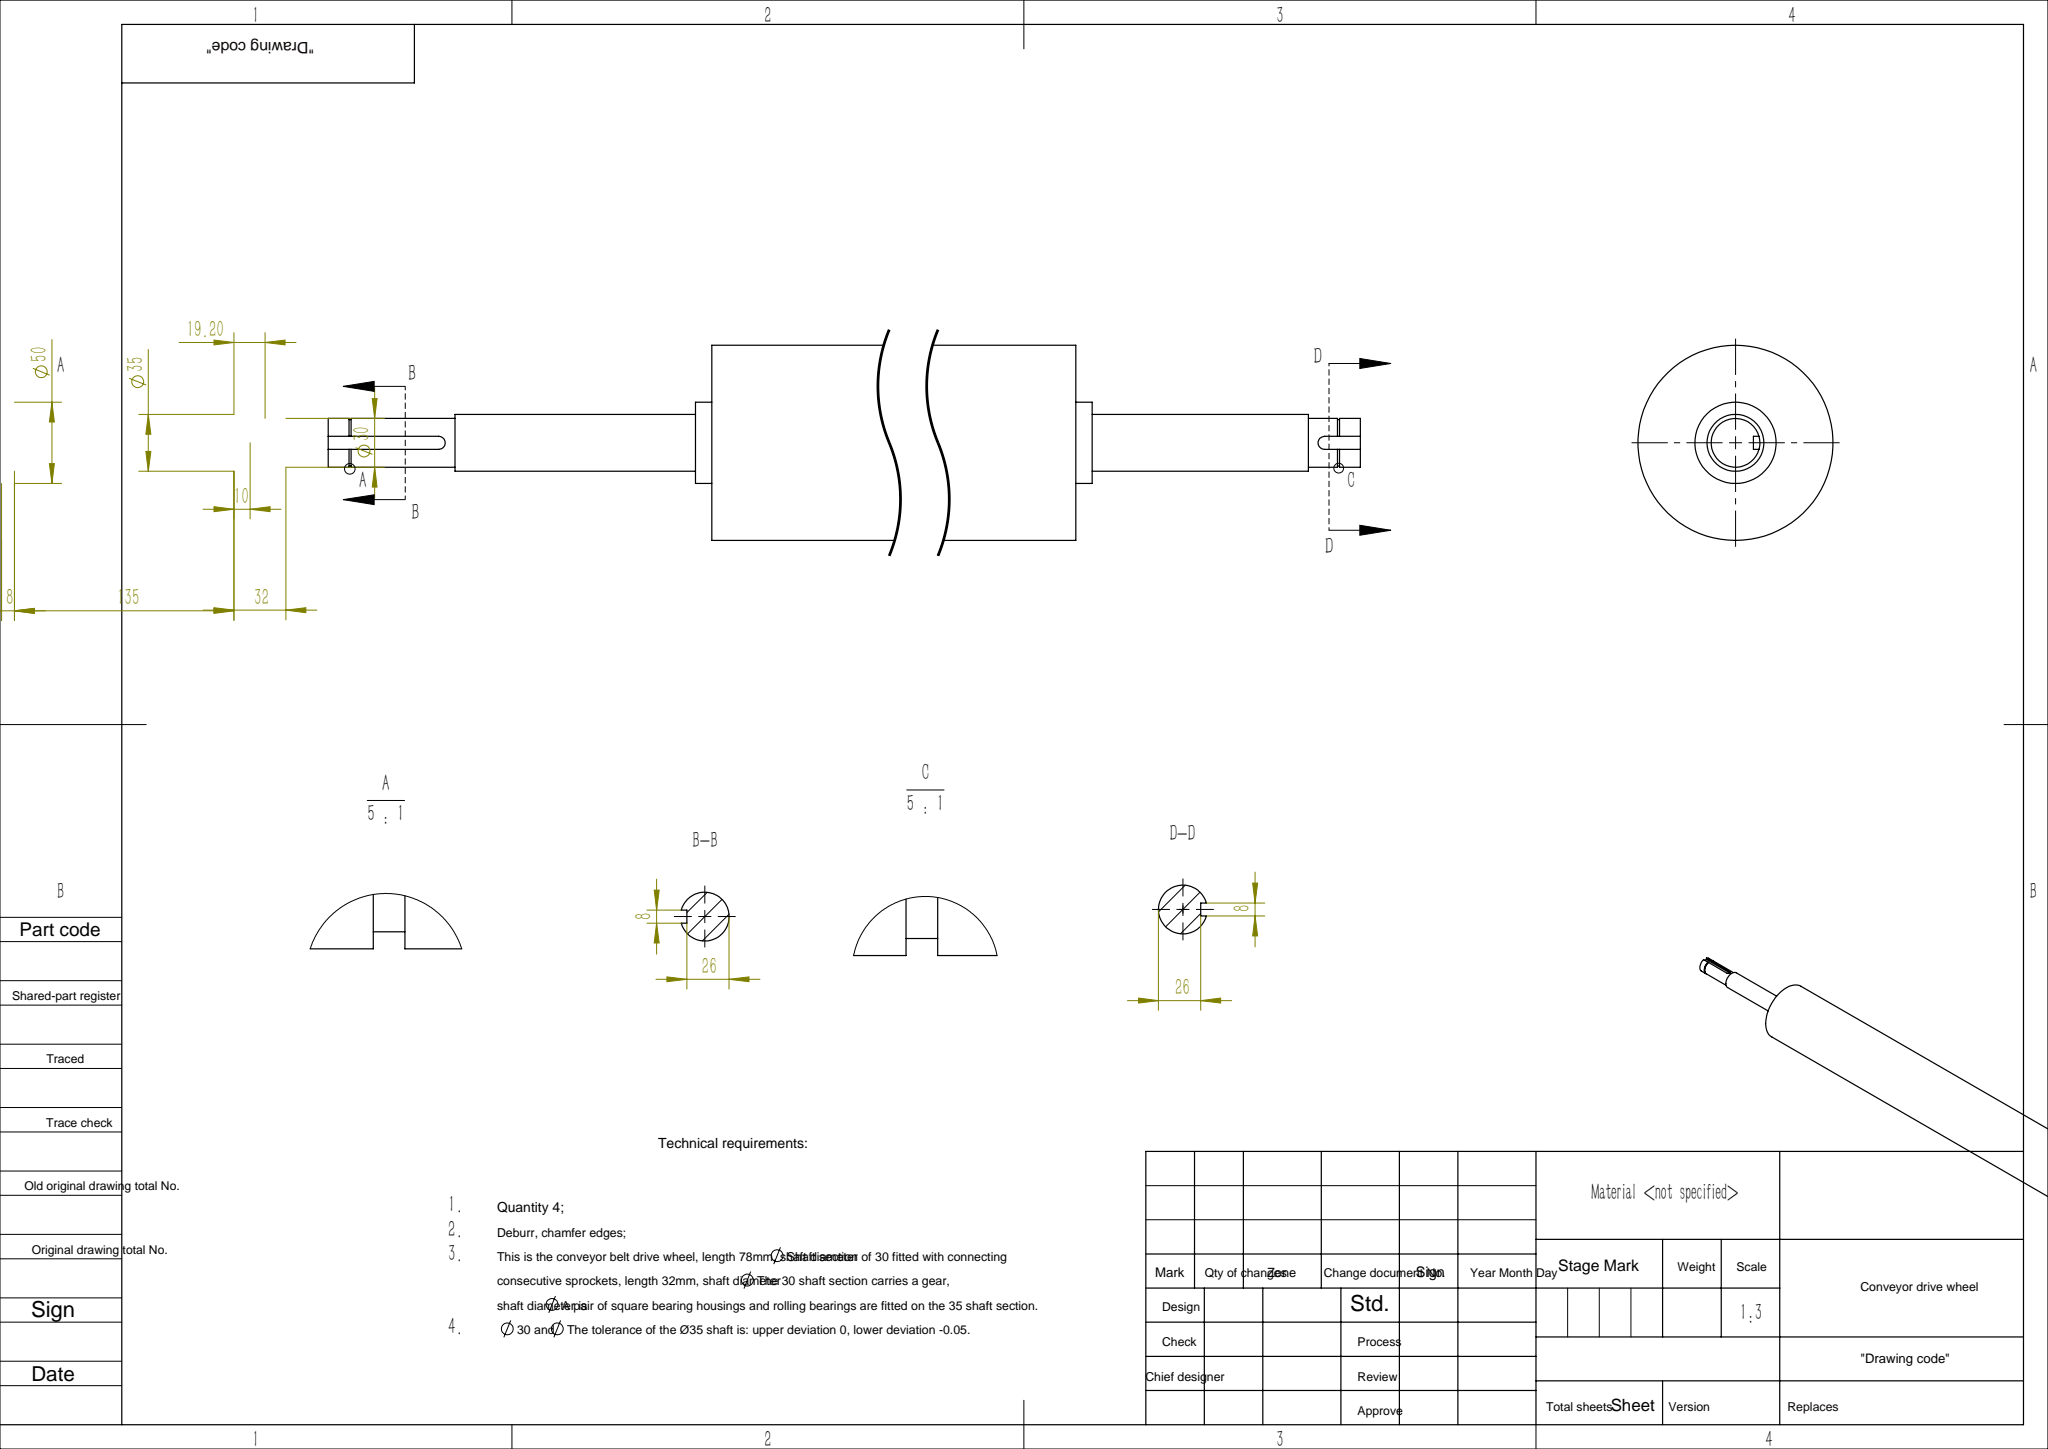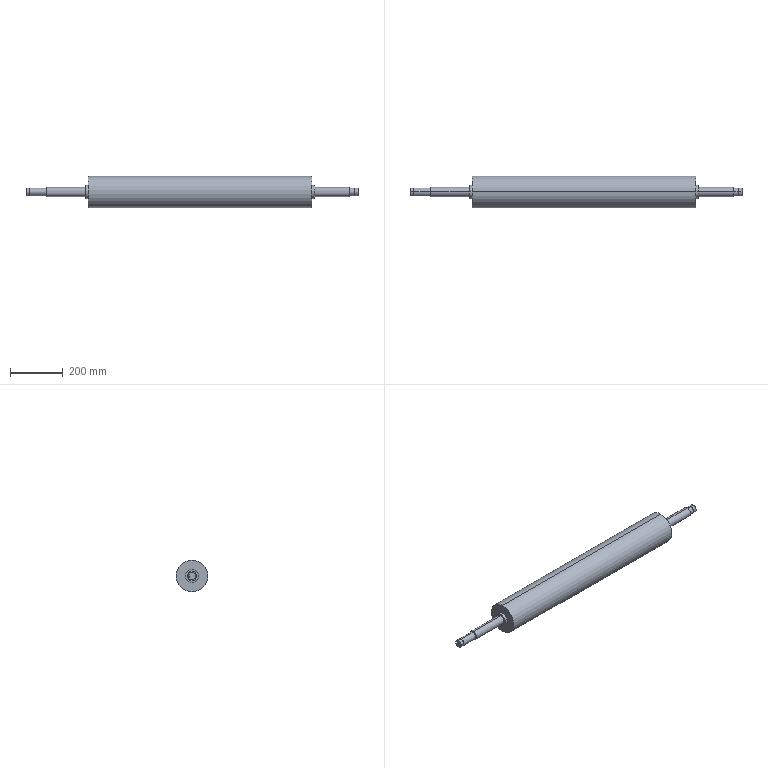Part | SolidWorks | features ICE 4, Revolution 1 | 1 solid | 46 faces | box 1261 x 120 x 120 mm | volume 9997554 mm3 | cylinder 28 | plane 18 | commonest cylinder face diameters 30 x10 28.6 x6 35 x4 50 x4 8 x2 120 x2